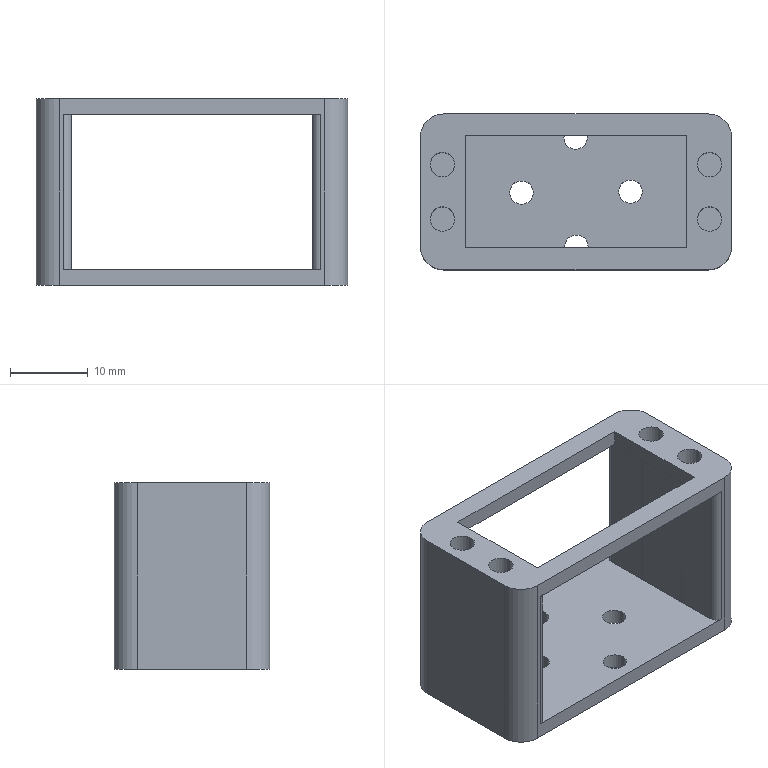Part | SolidWorks | features ICE 5, Fillet 2, Extrusion 1 | 1 solid | 42 faces | box 40 x 20 x 24 mm | volume 5034 mm3 | cylinder 24 | plane 18 | commonest cylinder face diameters 3 x8 3.15 x8 2 x4 6 x4
STEP:
#1=CARTESIAN_POINT('',(1.439,7.,-20.));
#2=VERTEX_POINT('',#1);
#3=CARTESIAN_POINT('',(-1.561,7.,-20.));
#4=VERTEX_POINT('',#3);
#5=CARTESIAN_POINT('',(-0.06094,7.,-20.));
#6=DIRECTION('',(0.,0.,-1.));
#7=DIRECTION('',(-1.,0.,0.));
#8=AXIS2_PLACEMENT_3D('',#5,#6,#7);
#9=CIRCLE('',#8,1.5);
#10=EDGE_CURVE('',#2,#4,#9,.T.);
#11=ORIENTED_EDGE('',*,*,#10,.F.);
#12=CARTESIAN_POINT('',(1.439,7.,-22.));
#13=VERTEX_POINT('',#12);
#14=CARTESIAN_POINT('',(1.439,7.,-20.));
#15=DIRECTION('',(0.,0.,-1.));
#16=VECTOR('',#15,1000.);
#17=LINE('',#14,#16);
#18=EDGE_CURVE('',#2,#13,#17,.T.);
#19=ORIENTED_EDGE('',*,*,#18,.T.);
#20=CARTESIAN_POINT('',(-1.561,7.,-22.));
#21=VERTEX_POINT('',#20);
#22=CARTESIAN_POINT('',(-0.06094,7.,-22.));
#23=DIRECTION('',(0.,0.,-1.));
#24=DIRECTION('',(-1.,0.,0.));
#25=AXIS2_PLACEMENT_3D('',#22,#23,#24);
#26=CIRCLE('',#25,1.5);
#27=EDGE_CURVE('',#13,#21,#26,.T.);
#28=ORIENTED_EDGE('',*,*,#27,.T.);
#29=CARTESIAN_POINT('',(-1.561,7.,-20.));
#30=DIRECTION('',(0.,0.,-1.));
#31=VECTOR('',#30,1000.);
#32=LINE('',#29,#31);
#33=EDGE_CURVE('',#4,#21,#32,.T.);
#34=ORIENTED_EDGE('',*,*,#33,.F.);
#35=EDGE_LOOP('',(#11,#19,#28,#34));
#36=FACE_OUTER_BOUND('',#35,.T.);
#37=CARTESIAN_POINT('',(-0.06094,7.,-20.));
#38=DIRECTION('',(0.,0.,-1.));
#39=DIRECTION('',(-1.,0.,0.));
#40=AXIS2_PLACEMENT_3D('',#37,#38,#39);
#41=CYLINDRICAL_SURFACE('',#40,1.5);
#42=ADVANCED_FACE('',(#36),#41,.F.);
#43=CARTESIAN_POINT('',(-5.5,-0.06094,-20.));
#44=VERTEX_POINT('',#43);
#45=CARTESIAN_POINT('',(-8.5,-0.06094,-20.));
#46=VERTEX_POINT('',#45);
#47=CARTESIAN_POINT('',(-7.,-0.06094,-20.));
#48=DIRECTION('',(0.,0.,-1.));
#49=DIRECTION('',(-1.,0.,0.));
#50=AXIS2_PLACEMENT_3D('',#47,#48,#49);
#51=CIRCLE('',#50,1.5);
#52=EDGE_CURVE('',#44,#46,#51,.T.);
#53=ORIENTED_EDGE('',*,*,#52,.F.);
#54=CARTESIAN_POINT('',(-5.5,-0.06094,-22.));
#55=VERTEX_POINT('',#54);
#56=CARTESIAN_POINT('',(-5.5,-0.06094,-20.));
#57=DIRECTION('',(0.,0.,-1.));
#58=VECTOR('',#57,1000.);
#59=LINE('',#56,#58);
#60=EDGE_CURVE('',#44,#55,#59,.T.);
#61=ORIENTED_EDGE('',*,*,#60,.T.);
#62=CARTESIAN_POINT('',(-8.5,-0.06094,-22.));
#63=VERTEX_POINT('',#62);
#64=CARTESIAN_POINT('',(-7.,-0.06094,-22.));
#65=DIRECTION('',(0.,0.,-1.));
#66=DIRECTION('',(-1.,0.,0.));
#67=AXIS2_PLACEMENT_3D('',#64,#65,#66);
#68=CIRCLE('',#67,1.5);
#69=EDGE_CURVE('',#55,#63,#68,.T.);
#70=ORIENTED_EDGE('',*,*,#69,.T.);
#71=CARTESIAN_POINT('',(-8.5,-0.06094,-20.));
#72=DIRECTION('',(0.,0.,-1.));
#73=VECTOR('',#72,1000.);
#74=LINE('',#71,#73);
#75=EDGE_CURVE('',#46,#63,#74,.T.);
#76=ORIENTED_EDGE('',*,*,#75,.F.);
#77=EDGE_LOOP('',(#53,#61,#70,#76));
#78=FACE_OUTER_BOUND('',#77,.T.);
#79=CARTESIAN_POINT('',(-7.,-0.06094,-20.));
#80=DIRECTION('',(0.,0.,-1.));
#81=DIRECTION('',(-1.,0.,0.));
#82=AXIS2_PLACEMENT_3D('',#79,#80,#81);
#83=CYLINDRICAL_SURFACE('',#82,1.5);
#84=ADVANCED_FACE('',(#78),#83,.F.);
#85=CARTESIAN_POINT('',(1.561,-7.,-20.));
#86=VERTEX_POINT('',#85);
#87=CARTESIAN_POINT('',(-1.439,-7.,-20.));
#88=VERTEX_POINT('',#87);
#89=CARTESIAN_POINT('',(0.06094,-7.,-20.));
#90=DIRECTION('',(0.,0.,-1.));
#91=DIRECTION('',(-1.,0.,0.));
#92=AXIS2_PLACEMENT_3D('',#89,#90,#91);
#93=CIRCLE('',#92,1.5);
#94=EDGE_CURVE('',#86,#88,#93,.T.);
#95=ORIENTED_EDGE('',*,*,#94,.F.);
#96=CARTESIAN_POINT('',(1.561,-7.,-22.));
#97=VERTEX_POINT('',#96);
#98=CARTESIAN_POINT('',(1.561,-7.,-20.));
#99=DIRECTION('',(0.,0.,-1.));
#100=VECTOR('',#99,1000.);
#101=LINE('',#98,#100);
#102=EDGE_CURVE('',#86,#97,#101,.T.);
#103=ORIENTED_EDGE('',*,*,#102,.T.);
#104=CARTESIAN_POINT('',(-1.439,-7.,-22.));
#105=VERTEX_POINT('',#104);
#106=CARTESIAN_POINT('',(0.06094,-7.,-22.));
#107=DIRECTION('',(0.,0.,-1.));
#108=DIRECTION('',(-1.,0.,0.));
#109=AXIS2_PLACEMENT_3D('',#106,#107,#108);
#110=CIRCLE('',#109,1.5);
#111=EDGE_CURVE('',#97,#105,#110,.T.);
#112=ORIENTED_EDGE('',*,*,#111,.T.);
#113=CARTESIAN_POINT('',(-1.439,-7.,-20.));
#114=DIRECTION('',(0.,0.,-1.));
#115=VECTOR('',#114,1000.);
#116=LINE('',#113,#115);
#117=EDGE_CURVE('',#88,#105,#116,.T.);
#118=ORIENTED_EDGE('',*,*,#117,.F.);
#119=EDGE_LOOP('',(#95,#103,#112,#118));
#120=FACE_OUTER_BOUND('',#119,.T.);
#121=CARTESIAN_POINT('',(0.06094,-7.,-20.));
#122=DIRECTION('',(0.,0.,-1.));
#123=DIRECTION('',(-1.,0.,0.));
#124=AXIS2_PLACEMENT_3D('',#121,#122,#123);
#125=CYLINDRICAL_SURFACE('',#124,1.5);
#126=ADVANCED_FACE('',(#120),#125,.F.);
#127=CARTESIAN_POINT('',(8.5,0.06094,-20.));
#128=VERTEX_POINT('',#127);
#129=CARTESIAN_POINT('',(5.5,0.06094,-20.));
#130=VERTEX_POINT('',#129);
#131=CARTESIAN_POINT('',(7.,0.06094,-20.));
#132=DIRECTION('',(0.,0.,-1.));
#133=DIRECTION('',(-1.,0.,0.));
#134=AXIS2_PLACEMENT_3D('',#131,#132,#133);
#135=CIRCLE('',#134,1.5);
#136=EDGE_CURVE('',#128,#130,#135,.T.);
#137=ORIENTED_EDGE('',*,*,#136,.F.);
#138=CARTESIAN_POINT('',(8.5,0.06094,-22.));
#139=VERTEX_POINT('',#138);
#140=CARTESIAN_POINT('',(8.5,0.06094,-20.));
#141=DIRECTION('',(0.,0.,-1.));
#142=VECTOR('',#141,1000.);
#143=LINE('',#140,#142);
#144=EDGE_CURVE('',#128,#139,#143,.T.);
#145=ORIENTED_EDGE('',*,*,#144,.T.);
#146=CARTESIAN_POINT('',(5.5,0.06094,-22.));
#147=VERTEX_POINT('',#146);
#148=CARTESIAN_POINT('',(7.,0.06094,-22.));
#149=DIRECTION('',(0.,0.,-1.));
#150=DIRECTION('',(-1.,0.,0.));
#151=AXIS2_PLACEMENT_3D('',#148,#149,#150);
#152=CIRCLE('',#151,1.5);
#153=EDGE_CURVE('',#139,#147,#152,.T.);
#154=ORIENTED_EDGE('',*,*,#153,.T.);
#155=CARTESIAN_POINT('',(5.5,0.06094,-20.));
#156=DIRECTION('',(0.,0.,-1.));
#157=VECTOR('',#156,1000.);
#158=LINE('',#155,#157);
#159=EDGE_CURVE('',#130,#147,#158,.T.);
#160=ORIENTED_EDGE('',*,*,#159,.F.);
#161=EDGE_LOOP('',(#137,#145,#154,#160));
#162=FACE_OUTER_BOUND('',#161,.T.);
#163=CARTESIAN_POINT('',(7.,0.06094,-20.));
#164=DIRECTION('',(0.,0.,-1.));
#165=DIRECTION('',(-1.,0.,0.));
#166=AXIS2_PLACEMENT_3D('',#163,#164,#165);
#167=CYLINDRICAL_SURFACE('',#166,1.5);
#168=ADVANCED_FACE('',(#162),#167,.F.);
#169=CARTESIAN_POINT('',(-18.725,-3.5,-20.));
#170=VERTEX_POINT('',#169);
#171=CARTESIAN_POINT('',(-15.575,-3.5,-20.));
#172=VERTEX_POINT('',#171);
#173=CARTESIAN_POINT('',(-17.15,-3.5,-20.));
#174=DIRECTION('',(0.,0.,1.));
#175=DIRECTION('',(-1.,0.,0.));
#176=AXIS2_PLACEMENT_3D('',#173,#174,#175);
#177=CIRCLE('',#176,1.575);
#178=EDGE_CURVE('',#170,#172,#177,.T.);
#179=ORIENTED_EDGE('',*,*,#178,.F.);
#180=CARTESIAN_POINT('',(-18.725,-3.5,2.));
#181=VERTEX_POINT('',#180);
#182=CARTESIAN_POINT('',(-18.725,-3.5,-4.));
#183=DIRECTION('',(0.,0.,1.));
#184=VECTOR('',#183,1000.);
#185=LINE('',#182,#184);
#186=EDGE_CURVE('',#170,#181,#185,.T.);
#187=ORIENTED_EDGE('',*,*,#186,.T.);
#188=CARTESIAN_POINT('',(-15.575,-3.5,2.));
#189=VERTEX_POINT('',#188);
#190=CARTESIAN_POINT('',(-17.15,-3.5,2.));
#191=DIRECTION('',(0.,0.,1.));
#192=DIRECTION('',(1.,0.,0.));
#193=AXIS2_PLACEMENT_3D('',#190,#191,#192);
#194=CIRCLE('',#193,1.575);
#195=EDGE_CURVE('',#181,#189,#194,.T.);
#196=ORIENTED_EDGE('',*,*,#195,.T.);
#197=CARTESIAN_POINT('',(-15.575,-3.5,-4.));
#198=DIRECTION('',(0.,0.,1.));
#199=VECTOR('',#198,1000.);
#200=LINE('',#197,#199);
#201=EDGE_CURVE('',#172,#189,#200,.T.);
#202=ORIENTED_EDGE('',*,*,#201,.F.);
#203=EDGE_LOOP('',(#179,#187,#196,#202));
#204=FACE_OUTER_BOUND('',#203,.T.);
#205=CARTESIAN_POINT('',(-17.15,-3.5,-4.));
#206=DIRECTION('',(0.,0.,1.));
#207=DIRECTION('',(1.,0.,0.));
#208=AXIS2_PLACEMENT_3D('',#205,#206,#207);
#209=CYLINDRICAL_SURFACE('',#208,1.575);
#210=ADVANCED_FACE('',(#204),#209,.F.);
#211=CARTESIAN_POINT('',(15.575,3.5,-20.));
#212=VERTEX_POINT('',#211);
#213=CARTESIAN_POINT('',(18.725,3.5,-20.));
#214=VERTEX_POINT('',#213);
#215=CARTESIAN_POINT('',(17.15,3.5,-20.));
#216=DIRECTION('',(0.,0.,1.));
#217=DIRECTION('',(-1.,0.,0.));
#218=AXIS2_PLACEMENT_3D('',#215,#216,#217);
#219=CIRCLE('',#218,1.575);
#220=EDGE_CURVE('',#212,#214,#219,.T.);
#221=ORIENTED_EDGE('',*,*,#220,.F.);
#222=CARTESIAN_POINT('',(15.575,3.5,2.));
#223=VERTEX_POINT('',#222);
#224=CARTESIAN_POINT('',(15.575,3.5,-4.));
#225=DIRECTION('',(0.,0.,1.));
#226=VECTOR('',#225,1000.);
#227=LINE('',#224,#226);
#228=EDGE_CURVE('',#212,#223,#227,.T.);
#229=ORIENTED_EDGE('',*,*,#228,.T.);
#230=CARTESIAN_POINT('',(18.725,3.5,2.));
#231=VERTEX_POINT('',#230);
#232=CARTESIAN_POINT('',(17.15,3.5,2.));
#233=DIRECTION('',(0.,0.,1.));
#234=DIRECTION('',(-1.,0.,0.));
#235=AXIS2_PLACEMENT_3D('',#232,#233,#234);
#236=CIRCLE('',#235,1.575);
#237=EDGE_CURVE('',#223,#231,#236,.T.);
#238=ORIENTED_EDGE('',*,*,#237,.T.);
#239=CARTESIAN_POINT('',(18.725,3.5,-4.));
#240=DIRECTION('',(0.,0.,1.));
#241=VECTOR('',#240,1000.);
#242=LINE('',#239,#241);
#243=EDGE_CURVE('',#214,#231,#242,.T.);
#244=ORIENTED_EDGE('',*,*,#243,.F.);
#245=EDGE_LOOP('',(#221,#229,#238,#244));
#246=FACE_OUTER_BOUND('',#245,.T.);
#247=CARTESIAN_POINT('',(17.15,3.5,-4.));
#248=DIRECTION('',(0.,0.,1.));
#249=DIRECTION('',(1.,0.,0.));
#250=AXIS2_PLACEMENT_3D('',#247,#248,#249);
#251=CYLINDRICAL_SURFACE('',#250,1.575);
#252=ADVANCED_FACE('',(#246),#251,.F.);
#253=CARTESIAN_POINT('',(15.575,-3.5,-20.));
#254=VERTEX_POINT('',#253);
#255=CARTESIAN_POINT('',(18.725,-3.5,-20.));
#256=VERTEX_POINT('',#255);
#257=CARTESIAN_POINT('',(17.15,-3.5,-20.));
#258=DIRECTION('',(0.,0.,1.));
#259=DIRECTION('',(-1.,0.,0.));
#260=AXIS2_PLACEMENT_3D('',#257,#258,#259);
#261=CIRCLE('',#260,1.575);
#262=EDGE_CURVE('',#254,#256,#261,.T.);
#263=ORIENTED_EDGE('',*,*,#262,.F.);
#264=CARTESIAN_POINT('',(15.575,-3.5,2.));
#265=VERTEX_POINT('',#264);
#266=CARTESIAN_POINT('',(15.575,-3.5,-4.));
#267=DIRECTION('',(0.,0.,1.));
#268=VECTOR('',#267,1000.);
#269=LINE('',#266,#268);
#270=EDGE_CURVE('',#254,#265,#269,.T.);
#271=ORIENTED_EDGE('',*,*,#270,.T.);
#272=CARTESIAN_POINT('',(18.725,-3.5,2.));
#273=VERTEX_POINT('',#272);
#274=CARTESIAN_POINT('',(17.15,-3.5,2.));
#275=DIRECTION('',(0.,0.,1.));
#276=DIRECTION('',(-1.,0.,0.));
#277=AXIS2_PLACEMENT_3D('',#274,#275,#276);
#278=CIRCLE('',#277,1.575);
#279=EDGE_CURVE('',#265,#273,#278,.T.);
#280=ORIENTED_EDGE('',*,*,#279,.T.);
#281=CARTESIAN_POINT('',(18.725,-3.5,-4.));
#282=DIRECTION('',(0.,0.,1.));
#283=VECTOR('',#282,1000.);
#284=LINE('',#281,#283);
#285=EDGE_CURVE('',#256,#273,#284,.T.);
#286=ORIENTED_EDGE('',*,*,#285,.F.);
#287=EDGE_LOOP('',(#263,#271,#280,#286));
#288=FACE_OUTER_BOUND('',#287,.T.);
#289=CARTESIAN_POINT('',(17.15,-3.5,-4.));
#290=DIRECTION('',(0.,0.,1.));
#291=DIRECTION('',(1.,0.,0.));
#292=AXIS2_PLACEMENT_3D('',#289,#290,#291);
#293=CYLINDRICAL_SURFACE('',#292,1.575);
#294=ADVANCED_FACE('',(#288),#293,.F.);
#295=CARTESIAN_POINT('',(-18.725,3.5,-20.));
#296=VERTEX_POINT('',#295);
#297=CARTESIAN_POINT('',(-15.575,3.5,-20.));
#298=VERTEX_POINT('',#297);
#299=CARTESIAN_POINT('',(-17.15,3.5,-20.));
#300=DIRECTION('',(0.,0.,1.));
#301=DIRECTION('',(-1.,0.,0.));
#302=AXIS2_PLACEMENT_3D('',#299,#300,#301);
#303=CIRCLE('',#302,1.575);
#304=EDGE_CURVE('',#296,#298,#303,.T.);
#305=ORIENTED_EDGE('',*,*,#304,.F.);
#306=CARTESIAN_POINT('',(-18.725,3.5,2.));
#307=VERTEX_POINT('',#306);
#308=CARTESIAN_POINT('',(-18.725,3.5,-4.));
#309=DIRECTION('',(0.,0.,1.));
#310=VECTOR('',#309,1000.);
#311=LINE('',#308,#310);
#312=EDGE_CURVE('',#296,#307,#311,.T.);
#313=ORIENTED_EDGE('',*,*,#312,.T.);
#314=CARTESIAN_POINT('',(-15.575,3.5,2.));
#315=VERTEX_POINT('',#314);
#316=CARTESIAN_POINT('',(-17.15,3.5,2.));
#317=DIRECTION('',(0.,0.,1.));
#318=DIRECTION('',(1.,0.,0.));
#319=AXIS2_PLACEMENT_3D('',#316,#317,#318);
#320=CIRCLE('',#319,1.575);
#321=EDGE_CURVE('',#307,#315,#320,.T.);
#322=ORIENTED_EDGE('',*,*,#321,.T.);
#323=CARTESIAN_POINT('',(-15.575,3.5,-4.));
#324=DIRECTION('',(0.,0.,1.));
#325=VECTOR('',#324,1000.);
#326=LINE('',#323,#325);
#327=EDGE_CURVE('',#298,#315,#326,.T.);
#328=ORIENTED_EDGE('',*,*,#327,.F.);
#329=EDGE_LOOP('',(#305,#313,#322,#328));
#330=FACE_OUTER_BOUND('',#329,.T.);
#331=CARTESIAN_POINT('',(-17.15,3.5,-4.));
#332=DIRECTION('',(0.,0.,1.));
#333=DIRECTION('',(1.,0.,0.));
#334=AXIS2_PLACEMENT_3D('',#331,#332,#333);
#335=CYLINDRICAL_SURFACE('',#334,1.575);
#336=ADVANCED_FACE('',(#330),#335,.F.);
#337=CARTESIAN_POINT('',(14.25,-7.2,0.));
#338=VERTEX_POINT('',#337);
#339=CARTESIAN_POINT('',(-14.25,-7.2,0.));
#340=VERTEX_POINT('',#339);
#341=CARTESIAN_POINT('',(0.,-7.2,0.));
#342=DIRECTION('',(-1.,0.,0.));
#343=VECTOR('',#342,1000.);
#344=LINE('',#341,#343);
#345=EDGE_CURVE('',#338,#340,#344,.T.);
#346=ORIENTED_EDGE('',*,*,#345,.F.);
#347=CARTESIAN_POINT('',(14.25,7.2,0.));
#348=VERTEX_POINT('',#347);
#349=CARTESIAN_POINT('',(14.25,0.,0.));
#350=DIRECTION('',(0.,-1.,0.));
#351=VECTOR('',#350,1000.);
#352=LINE('',#349,#351);
#353=EDGE_CURVE('',#348,#338,#352,.T.);
#354=ORIENTED_EDGE('',*,*,#353,.F.);
#355=CARTESIAN_POINT('',(-14.25,7.2,0.));
#356=VERTEX_POINT('',#355);
#357=CARTESIAN_POINT('',(0.,7.2,0.));
#358=DIRECTION('',(-1.,0.,0.));
#359=VECTOR('',#358,1000.);
#360=LINE('',#357,#359);
#361=EDGE_CURVE('',#348,#356,#360,.T.);
#362=ORIENTED_EDGE('',*,*,#361,.T.);
#363=CARTESIAN_POINT('',(-14.25,0.,0.));
#364=DIRECTION('',(0.,-1.,0.));
#365=VECTOR('',#364,1000.);
#366=LINE('',#363,#365);
#367=EDGE_CURVE('',#356,#340,#366,.T.);
#368=ORIENTED_EDGE('',*,*,#367,.T.);
#369=EDGE_LOOP('',(#346,#354,#362,#368));
#370=FACE_BOUND('',#369,.T.);
#371=CARTESIAN_POINT('',(16.5,10.,0.));
#372=VERTEX_POINT('',#371);
#373=CARTESIAN_POINT('',(-16.5,10.,0.));
#374=VERTEX_POINT('',#373);
#375=CARTESIAN_POINT('',(-20.,10.,0.));
#376=DIRECTION('',(-1.,0.,0.));
#377=VECTOR('',#376,1000.);
#378=LINE('',#375,#377);
#379=EDGE_CURVE('',#372,#374,#378,.T.);
#380=ORIENTED_EDGE('',*,*,#379,.F.);
#381=CARTESIAN_POINT('',(15.5,9.,0.));
#382=VERTEX_POINT('',#381);
#383=CARTESIAN_POINT('',(16.5,9.,0.));
#384=DIRECTION('',(0.,0.,1.));
#385=DIRECTION('',(-1.,0.,0.));
#386=AXIS2_PLACEMENT_3D('',#383,#384,#385);
#387=CIRCLE('',#386,1.);
#388=EDGE_CURVE('',#372,#382,#387,.T.);
#389=ORIENTED_EDGE('',*,*,#388,.T.);
#390=CARTESIAN_POINT('',(15.5,-9.,0.));
#391=VERTEX_POINT('',#390);
#392=CARTESIAN_POINT('',(15.5,0.,0.));
#393=DIRECTION('',(0.,1.,0.));
#394=VECTOR('',#393,1000.);
#395=LINE('',#392,#394);
#396=EDGE_CURVE('',#391,#382,#395,.T.);
#397=ORIENTED_EDGE('',*,*,#396,.F.);
#398=CARTESIAN_POINT('',(16.5,-10.,0.));
#399=VERTEX_POINT('',#398);
#400=CARTESIAN_POINT('',(16.5,-9.,0.));
#401=DIRECTION('',(0.,0.,1.));
#402=DIRECTION('',(-1.,0.,0.));
#403=AXIS2_PLACEMENT_3D('',#400,#401,#402);
#404=CIRCLE('',#403,1.);
#405=EDGE_CURVE('',#391,#399,#404,.T.);
#406=ORIENTED_EDGE('',*,*,#405,.T.);
#407=CARTESIAN_POINT('',(-16.5,-10.,0.));
#408=VERTEX_POINT('',#407);
#409=CARTESIAN_POINT('',(-20.,-10.,0.));
#410=DIRECTION('',(1.,0.,0.));
#411=VECTOR('',#410,1000.);
#412=LINE('',#409,#411);
#413=EDGE_CURVE('',#408,#399,#412,.T.);
#414=ORIENTED_EDGE('',*,*,#413,.F.);
#415=CARTESIAN_POINT('',(-15.5,-9.,0.));
#416=VERTEX_POINT('',#415);
#417=CARTESIAN_POINT('',(-16.5,-9.,0.));
#418=DIRECTION('',(0.,0.,1.));
#419=DIRECTION('',(-1.,0.,0.));
#420=AXIS2_PLACEMENT_3D('',#417,#418,#419);
#421=CIRCLE('',#420,1.);
#422=EDGE_CURVE('',#408,#416,#421,.T.);
#423=ORIENTED_EDGE('',*,*,#422,.T.);
#424=CARTESIAN_POINT('',(-15.5,9.,0.));
#425=VERTEX_POINT('',#424);
#426=CARTESIAN_POINT('',(-15.5,0.,0.));
#427=DIRECTION('',(0.,1.,0.));
#428=VECTOR('',#427,1000.);
#429=LINE('',#426,#428);
#430=EDGE_CURVE('',#416,#425,#429,.T.);
#431=ORIENTED_EDGE('',*,*,#430,.T.);
#432=CARTESIAN_POINT('',(-16.5,9.,0.));
#433=DIRECTION('',(0.,0.,1.));
#434=DIRECTION('',(-1.,0.,0.));
#435=AXIS2_PLACEMENT_3D('',#432,#433,#434);
#436=CIRCLE('',#435,1.);
#437=EDGE_CURVE('',#425,#374,#436,.T.);
#438=ORIENTED_EDGE('',*,*,#437,.T.);
#439=EDGE_LOOP('',(#380,#389,#397,#406,#414,#423,#431,#438));
#440=FACE_OUTER_BOUND('',#439,.T.);
#441=CARTESIAN_POINT('',(0.,0.,0.));
#442=DIRECTION('',(0.,0.,-1.));
#443=DIRECTION('',(-1.,0.,0.));
#444=AXIS2_PLACEMENT_3D('',#441,#442,#443);
#445=PLANE('',#444);
#446=ADVANCED_FACE('',(#370,#440),#445,.T.);
#447=CARTESIAN_POINT('',(20.,-7.,2.));
#448=VERTEX_POINT('',#447);
#449=CARTESIAN_POINT('',(20.,7.,2.));
#450=VERTEX_POINT('',#449);
#451=CARTESIAN_POINT('',(20.,-10.,2.));
#452=DIRECTION('',(0.,1.,0.));
#453=VECTOR('',#452,1000.);
#454=LINE('',#451,#453);
#455=EDGE_CURVE('',#448,#450,#454,.T.);
#456=ORIENTED_EDGE('',*,*,#455,.F.);
#457=CARTESIAN_POINT('',(20.,-7.,-22.));
#458=VERTEX_POINT('',#457);
#459=CARTESIAN_POINT('',(20.,-7.,2.));
#460=DIRECTION('',(0.,0.,-1.));
#461=VECTOR('',#460,1000.);
#462=LINE('',#459,#461);
#463=EDGE_CURVE('',#448,#458,#462,.T.);
#464=ORIENTED_EDGE('',*,*,#463,.T.);
#465=CARTESIAN_POINT('',(20.,7.,-22.));
#466=VERTEX_POINT('',#465);
#467=CARTESIAN_POINT('',(20.,10.,-22.));
#468=DIRECTION('',(0.,-1.,0.));
#469=VECTOR('',#468,1000.);
#470=LINE('',#467,#469);
#471=EDGE_CURVE('',#466,#458,#470,.T.);
#472=ORIENTED_EDGE('',*,*,#471,.F.);
#473=CARTESIAN_POINT('',(20.,7.,2.));
#474=DIRECTION('',(0.,0.,1.));
#475=VECTOR('',#474,1000.);
#476=LINE('',#473,#475);
#477=EDGE_CURVE('',#466,#450,#476,.T.);
#478=ORIENTED_EDGE('',*,*,#477,.T.);
#479=EDGE_LOOP('',(#456,#464,#472,#478));
#480=FACE_OUTER_BOUND('',#479,.T.);
#481=CARTESIAN_POINT('',(20.,-10.,2.));
#482=DIRECTION('',(-1.,0.,0.));
#483=DIRECTION('',(0.,0.,1.));
#484=AXIS2_PLACEMENT_3D('',#481,#482,#483);
#485=PLANE('',#484);
#486=ADVANCED_FACE('',(#480),#485,.F.);
#487=ORIENTED_EDGE('',*,*,#379,.T.);
#488=CARTESIAN_POINT('',(-16.5,10.,-20.));
#489=VERTEX_POINT('',#488);
#490=CARTESIAN_POINT('',(-16.5,10.,-20.));
#491=DIRECTION('',(0.,0.,-1.));
#492=VECTOR('',#491,1000.);
#493=LINE('',#490,#492);
#494=EDGE_CURVE('',#374,#489,#493,.T.);
#495=ORIENTED_EDGE('',*,*,#494,.T.);
#496=CARTESIAN_POINT('',(16.5,10.,-20.));
#497=VERTEX_POINT('',#496);
#498=CARTESIAN_POINT('',(20.,10.,-20.));
#499=DIRECTION('',(1.,0.,0.));
#500=VECTOR('',#499,1000.);
#501=LINE('',#498,#500);
#502=EDGE_CURVE('',#489,#497,#501,.T.);
#503=ORIENTED_EDGE('',*,*,#502,.T.);
#504=CARTESIAN_POINT('',(16.5,10.,2.));
#505=DIRECTION('',(0.,0.,1.));
#506=VECTOR('',#505,1000.);
#507=LINE('',#504,#506);
#508=EDGE_CURVE('',#497,#372,#507,.T.);
#509=ORIENTED_EDGE('',*,*,#508,.T.);
#510=EDGE_LOOP('',(#487,#495,#503,#509));
#511=FACE_BOUND('',#510,.T.);
#512=CARTESIAN_POINT('',(-17.,10.,-22.));
#513=VERTEX_POINT('',#512);
#514=CARTESIAN_POINT('',(17.,10.,-22.));
#515=VERTEX_POINT('',#514);
#516=CARTESIAN_POINT('',(20.,10.,-22.));
#517=DIRECTION('',(1.,0.,0.));
#518=VECTOR('',#517,1000.);
#519=LINE('',#516,#518);
#520=EDGE_CURVE('',#513,#515,#519,.T.);
#521=ORIENTED_EDGE('',*,*,#520,.F.);
#522=CARTESIAN_POINT('',(-17.,10.,2.));
#523=VERTEX_POINT('',#522);
#524=CARTESIAN_POINT('',(-17.,10.,2.));
#525=DIRECTION('',(0.,0.,1.));
#526=VECTOR('',#525,1000.);
#527=LINE('',#524,#526);
#528=EDGE_CURVE('',#513,#523,#527,.T.);
#529=ORIENTED_EDGE('',*,*,#528,.T.);
#530=CARTESIAN_POINT('',(17.,10.,2.));
#531=VERTEX_POINT('',#530);
#532=CARTESIAN_POINT('',(-20.,10.,2.));
#533=DIRECTION('',(-1.,0.,0.));
#534=VECTOR('',#533,1000.);
#535=LINE('',#532,#534);
#536=EDGE_CURVE('',#531,#523,#535,.T.);
#537=ORIENTED_EDGE('',*,*,#536,.F.);
#538=CARTESIAN_POINT('',(17.,10.,2.));
#539=DIRECTION('',(0.,0.,-1.));
#540=VECTOR('',#539,1000.);
#541=LINE('',#538,#540);
#542=EDGE_CURVE('',#531,#515,#541,.T.);
#543=ORIENTED_EDGE('',*,*,#542,.T.);
#544=EDGE_LOOP('',(#521,#529,#537,#543));
#545=FACE_OUTER_BOUND('',#544,.T.);
#546=CARTESIAN_POINT('',(-20.,10.,2.));
#547=DIRECTION('',(0.,-1.,0.));
#548=DIRECTION('',(0.,0.,-1.));
#549=AXIS2_PLACEMENT_3D('',#546,#547,#548);
#550=PLANE('',#549);
#551=ADVANCED_FACE('',(#511,#545),#550,.F.);
#552=CARTESIAN_POINT('',(-20.,7.,2.));
#553=VERTEX_POINT('',#552);
#554=CARTESIAN_POINT('',(-20.,-7.,2.));
#555=VERTEX_POINT('',#554);
#556=CARTESIAN_POINT('',(-20.,-10.,2.));
#557=DIRECTION('',(0.,-1.,0.));
#558=VECTOR('',#557,1000.);
#559=LINE('',#556,#558);
#560=EDGE_CURVE('',#553,#555,#559,.T.);
#561=ORIENTED_EDGE('',*,*,#560,.F.);
#562=CARTESIAN_POINT('',(-20.,7.,-22.));
#563=VERTEX_POINT('',#562);
#564=CARTESIAN_POINT('',(-20.,7.,2.));
#565=DIRECTION('',(0.,0.,-1.));
#566=VECTOR('',#565,1000.);
#567=LINE('',#564,#566);
#568=EDGE_CURVE('',#553,#563,#567,.T.);
#569=ORIENTED_EDGE('',*,*,#568,.T.);
#570=CARTESIAN_POINT('',(-20.,-7.,-22.));
#571=VERTEX_POINT('',#570);
#572=CARTESIAN_POINT('',(-20.,10.,-22.));
#573=DIRECTION('',(0.,1.,0.));
#574=VECTOR('',#573,1000.);
#575=LINE('',#572,#574);
#576=EDGE_CURVE('',#571,#563,#575,.T.);
#577=ORIENTED_EDGE('',*,*,#576,.F.);
#578=CARTESIAN_POINT('',(-20.,-7.,2.));
#579=DIRECTION('',(0.,0.,1.));
#580=VECTOR('',#579,1000.);
#581=LINE('',#578,#580);
#582=EDGE_CURVE('',#571,#555,#581,.T.);
#583=ORIENTED_EDGE('',*,*,#582,.T.);
#584=EDGE_LOOP('',(#561,#569,#577,#583));
#585=FACE_OUTER_BOUND('',#584,.T.);
#586=CARTESIAN_POINT('',(-20.,-10.,2.));
#587=DIRECTION('',(1.,0.,0.));
#588=DIRECTION('',(0.,0.,-1.));
#589=AXIS2_PLACEMENT_3D('',#586,#587,#588);
#590=PLANE('',#589);
#591=ADVANCED_FACE('',(#585),#590,.F.);
#592=CARTESIAN_POINT('',(-17.,-10.,2.));
#593=VERTEX_POINT('',#592);
#594=CARTESIAN_POINT('',(17.,-10.,2.));
#595=VERTEX_POINT('',#594);
#596=CARTESIAN_POINT('',(-20.,-10.,2.));
#597=DIRECTION('',(1.,0.,0.));
#598=VECTOR('',#597,1000.);
#599=LINE('',#596,#598);
#600=EDGE_CURVE('',#593,#595,#599,.T.);
#601=ORIENTED_EDGE('',*,*,#600,.F.);
#602=CARTESIAN_POINT('',(-17.,-10.,-22.));
#603=VERTEX_POINT('',#602);
#604=CARTESIAN_POINT('',(-17.,-10.,2.));
#605=DIRECTION('',(0.,0.,-1.));
#606=VECTOR('',#605,1000.);
#607=LINE('',#604,#606);
#608=EDGE_CURVE('',#593,#603,#607,.T.);
#609=ORIENTED_EDGE('',*,*,#608,.T.);
#610=CARTESIAN_POINT('',(17.,-10.,-22.));
#611=VERTEX_POINT('',#610);
#612=CARTESIAN_POINT('',(20.,-10.,-22.));
#613=DIRECTION('',(-1.,0.,0.));
#614=VECTOR('',#613,1000.);
#615=LINE('',#612,#614);
#616=EDGE_CURVE('',#611,#603,#615,.T.);
#617=ORIENTED_EDGE('',*,*,#616,.F.);
#618=CARTESIAN_POINT('',(17.,-10.,2.));
#619=DIRECTION('',(0.,0.,1.));
#620=VECTOR('',#619,1000.);
#621=LINE('',#618,#620);
#622=EDGE_CURVE('',#611,#595,#621,.T.);
#623=ORIENTED_EDGE('',*,*,#622,.T.);
#624=EDGE_LOOP('',(#601,#609,#617,#623));
#625=FACE_OUTER_BOUND('',#624,.T.);
#626=CARTESIAN_POINT('',(-16.5,-10.,-20.));
#627=VERTEX_POINT('',#626);
#628=CARTESIAN_POINT('',(-16.5,-10.,0.));
#629=DIRECTION('',(0.,0.,1.));
#630=VECTOR('',#629,1000.);
#631=LINE('',#628,#630);
#632=EDGE_CURVE('',#627,#408,#631,.T.);
#633=ORIENTED_EDGE('',*,*,#632,.T.);
#634=ORIENTED_EDGE('',*,*,#413,.T.);
#635=CARTESIAN_POINT('',(16.5,-10.,-20.));
#636=VERTEX_POINT('',#635);
#637=CARTESIAN_POINT('',(16.5,-10.,2.));
#638=DIRECTION('',(0.,0.,-1.));
#639=VECTOR('',#638,1000.);
#640=LINE('',#637,#639);
#641=EDGE_CURVE('',#399,#636,#640,.T.);
#642=ORIENTED_EDGE('',*,*,#641,.T.);
#643=CARTESIAN_POINT('',(20.,-10.,-20.));
#644=DIRECTION('',(-1.,0.,0.));
#645=VECTOR('',#644,1000.);
#646=LINE('',#643,#645);
#647=EDGE_CURVE('',#636,#627,#646,.T.);
#648=ORIENTED_EDGE('',*,*,#647,.T.);
#649=EDGE_LOOP('',(#633,#634,#642,#648));
#650=FACE_BOUND('',#649,.T.);
#651=CARTESIAN_POINT('',(-20.,-10.,2.));
#652=DIRECTION('',(0.,1.,0.));
#653=DIRECTION('',(0.,0.,1.));
#654=AXIS2_PLACEMENT_3D('',#651,#652,#653);
#655=PLANE('',#654);
#656=ADVANCED_FACE('',(#625,#650),#655,.F.);
#657=CARTESIAN_POINT('',(-17.15,-3.5,2.));
#658=DIRECTION('',(0.,0.,1.));
#659=DIRECTION('',(1.,0.,0.));
#660=AXIS2_PLACEMENT_3D('',#657,#658,#659);
#661=CIRCLE('',#660,1.575);
#662=EDGE_CURVE('',#189,#181,#661,.T.);
#663=ORIENTED_EDGE('',*,*,#662,.F.);
#664=ORIENTED_EDGE('',*,*,#195,.F.);
#665=EDGE_LOOP('',(#663,#664));
#666=FACE_BOUND('',#665,.T.);
#667=CARTESIAN_POINT('',(17.15,3.5,2.));
#668=DIRECTION('',(0.,0.,1.));
#669=DIRECTION('',(-1.,0.,0.));
#670=AXIS2_PLACEMENT_3D('',#667,#668,#669);
#671=CIRCLE('',#670,1.575);
#672=EDGE_CURVE('',#231,#223,#671,.T.);
#673=ORIENTED_EDGE('',*,*,#672,.F.);
#674=ORIENTED_EDGE('',*,*,#237,.F.);
#675=EDGE_LOOP('',(#673,#674));
#676=FACE_BOUND('',#675,.T.);
#677=CARTESIAN_POINT('',(17.15,-3.5,2.));
#678=DIRECTION('',(0.,0.,1.));
#679=DIRECTION('',(-1.,0.,0.));
#680=AXIS2_PLACEMENT_3D('',#677,#678,#679);
#681=CIRCLE('',#680,1.575);
#682=EDGE_CURVE('',#273,#265,#681,.T.);
#683=ORIENTED_EDGE('',*,*,#682,.F.);
#684=ORIENTED_EDGE('',*,*,#279,.F.);
#685=EDGE_LOOP('',(#683,#684));
#686=FACE_BOUND('',#685,.T.);
#687=CARTESIAN_POINT('',(-17.15,3.5,2.));
#688=DIRECTION('',(0.,0.,1.));
#689=DIRECTION('',(1.,0.,0.));
#690=AXIS2_PLACEMENT_3D('',#687,#688,#689);
#691=CIRCLE('',#690,1.575);
#692=EDGE_CURVE('',#315,#307,#691,.T.);
#693=ORIENTED_EDGE('',*,*,#692,.F.);
#694=ORIENTED_EDGE('',*,*,#321,.F.);
#695=EDGE_LOOP('',(#693,#694));
#696=FACE_BOUND('',#695,.T.);
#697=CARTESIAN_POINT('',(14.25,-7.2,2.));
#698=VERTEX_POINT('',#697);
#699=CARTESIAN_POINT('',(14.25,7.2,2.));
#700=VERTEX_POINT('',#699);
#701=CARTESIAN_POINT('',(14.25,-7.2,2.));
#702=DIRECTION('',(0.,1.,0.));
#703=VECTOR('',#702,1000.);
#704=LINE('',#701,#703);
#705=EDGE_CURVE('',#698,#700,#704,.T.);
#706=ORIENTED_EDGE('',*,*,#705,.F.);
#707=CARTESIAN_POINT('',(-14.25,-7.2,2.));
#708=VERTEX_POINT('',#707);
#709=CARTESIAN_POINT('',(-14.25,-7.2,2.));
#710=DIRECTION('',(1.,0.,0.));
#711=VECTOR('',#710,1000.);
#712=LINE('',#709,#711);
#713=EDGE_CURVE('',#708,#698,#712,.T.);
#714=ORIENTED_EDGE('',*,*,#713,.F.);
#715=CARTESIAN_POINT('',(-14.25,7.2,2.));
#716=VERTEX_POINT('',#715);
#717=CARTESIAN_POINT('',(-14.25,-7.2,2.));
#718=DIRECTION('',(0.,1.,0.));
#719=VECTOR('',#718,1000.);
#720=LINE('',#717,#719);
#721=EDGE_CURVE('',#708,#716,#720,.T.);
#722=ORIENTED_EDGE('',*,*,#721,.T.);
#723=CARTESIAN_POINT('',(-14.25,7.2,2.));
#724=DIRECTION('',(1.,0.,0.));
#725=VECTOR('',#724,1000.);
#726=LINE('',#723,#725);
#727=EDGE_CURVE('',#716,#700,#726,.T.);
#728=ORIENTED_EDGE('',*,*,#727,.T.);
#729=EDGE_LOOP('',(#706,#714,#722,#728));
#730=FACE_BOUND('',#729,.T.);
#731=ORIENTED_EDGE('',*,*,#536,.T.);
#732=CARTESIAN_POINT('',(-17.,7.,2.));
#733=DIRECTION('',(0.,0.,1.));
#734=DIRECTION('',(-1.,0.,0.));
#735=AXIS2_PLACEMENT_3D('',#732,#733,#734);
#736=CIRCLE('',#735,3.);
#737=EDGE_CURVE('',#523,#553,#736,.T.);
#738=ORIENTED_EDGE('',*,*,#737,.T.);
#739=ORIENTED_EDGE('',*,*,#560,.T.);
#740=CARTESIAN_POINT('',(-17.,-7.,2.));
#741=DIRECTION('',(0.,0.,1.));
#742=DIRECTION('',(-1.,0.,0.));
#743=AXIS2_PLACEMENT_3D('',#740,#741,#742);
#744=CIRCLE('',#743,3.);
#745=EDGE_CURVE('',#555,#593,#744,.T.);
#746=ORIENTED_EDGE('',*,*,#745,.T.);
#747=ORIENTED_EDGE('',*,*,#600,.T.);
#748=CARTESIAN_POINT('',(17.,-7.,2.));
#749=DIRECTION('',(0.,0.,1.));
#750=DIRECTION('',(-1.,0.,0.));
#751=AXIS2_PLACEMENT_3D('',#748,#749,#750);
#752=CIRCLE('',#751,3.);
#753=EDGE_CURVE('',#595,#448,#752,.T.);
#754=ORIENTED_EDGE('',*,*,#753,.T.);
#755=ORIENTED_EDGE('',*,*,#455,.T.);
#756=CARTESIAN_POINT('',(17.,7.,2.));
#757=DIRECTION('',(0.,0.,1.));
#758=DIRECTION('',(-1.,0.,0.));
#759=AXIS2_PLACEMENT_3D('',#756,#757,#758);
#760=CIRCLE('',#759,3.);
#761=EDGE_CURVE('',#450,#531,#760,.T.);
#762=ORIENTED_EDGE('',*,*,#761,.T.);
#763=EDGE_LOOP('',(#731,#738,#739,#746,#747,#754,#755,#762));
#764=FACE_OUTER_BOUND('',#763,.T.);
#765=CARTESIAN_POINT('',(0.,0.,2.));
#766=DIRECTION('',(0.,0.,-1.));
#767=DIRECTION('',(-1.,0.,0.));
#768=AXIS2_PLACEMENT_3D('',#765,#766,#767);
#769=PLANE('',#768);
#770=ADVANCED_FACE('',(#666,#676,#686,#696,#730,#764),#769,.F.);
#771=ORIENTED_EDGE('',*,*,#345,.T.);
#772=CARTESIAN_POINT('',(-14.25,-7.2,-4.));
#773=DIRECTION('',(0.,0.,1.));
#774=VECTOR('',#773,1000.);
#775=LINE('',#772,#774);
#776=EDGE_CURVE('',#340,#708,#775,.T.);
#777=ORIENTED_EDGE('',*,*,#776,.T.);
#778=ORIENTED_EDGE('',*,*,#713,.T.);
#779=CARTESIAN_POINT('',(14.25,-7.2,-4.));
#780=DIRECTION('',(0.,0.,1.));
#781=VECTOR('',#780,1000.);
#782=LINE('',#779,#781);
#783=EDGE_CURVE('',#338,#698,#782,.T.);
#784=ORIENTED_EDGE('',*,*,#783,.F.);
#785=EDGE_LOOP('',(#771,#777,#778,#784));
#786=FACE_OUTER_BOUND('',#785,.T.);
#787=CARTESIAN_POINT('',(-14.25,-7.2,-4.));
#788=DIRECTION('',(0.,-1.,0.));
#789=DIRECTION('',(0.,0.,-1.));
#790=AXIS2_PLACEMENT_3D('',#787,#788,#789);
#791=PLANE('',#790);
#792=ADVANCED_FACE('',(#786),#791,.F.);
#793=CARTESIAN_POINT('',(-14.25,7.2,-4.));
#794=DIRECTION('',(0.,0.,1.));
#795=VECTOR('',#794,1000.);
#796=LINE('',#793,#795);
#797=EDGE_CURVE('',#356,#716,#796,.T.);
#798=ORIENTED_EDGE('',*,*,#797,.T.);
#799=ORIENTED_EDGE('',*,*,#721,.F.);
#800=ORIENTED_EDGE('',*,*,#776,.F.);
#801=ORIENTED_EDGE('',*,*,#367,.F.);
#802=EDGE_LOOP('',(#798,#799,#800,#801));
#803=FACE_OUTER_BOUND('',#802,.T.);
#804=CARTESIAN_POINT('',(-14.25,-7.2,-4.));
#805=DIRECTION('',(1.,0.,0.));
#806=DIRECTION('',(0.,0.,-1.));
#807=AXIS2_PLACEMENT_3D('',#804,#805,#806);
#808=PLANE('',#807);
#809=ADVANCED_FACE('',(#803),#808,.T.);
#810=CARTESIAN_POINT('',(14.25,7.2,-4.));
#811=DIRECTION('',(0.,0.,1.));
#812=VECTOR('',#811,1000.);
#813=LINE('',#810,#812);
#814=EDGE_CURVE('',#348,#700,#813,.T.);
#815=ORIENTED_EDGE('',*,*,#814,.T.);
#816=ORIENTED_EDGE('',*,*,#727,.F.);
#817=ORIENTED_EDGE('',*,*,#797,.F.);
#818=ORIENTED_EDGE('',*,*,#361,.F.);
#819=EDGE_LOOP('',(#815,#816,#817,#818));
#820=FACE_OUTER_BOUND('',#819,.T.);
#821=CARTESIAN_POINT('',(-14.25,7.2,-4.));
#822=DIRECTION('',(0.,-1.,0.));
#823=DIRECTION('',(0.,0.,-1.));
#824=AXIS2_PLACEMENT_3D('',#821,#822,#823);
#825=PLANE('',#824);
#826=ADVANCED_FACE('',(#820),#825,.T.);
#827=ORIENTED_EDGE('',*,*,#353,.T.);
#828=ORIENTED_EDGE('',*,*,#783,.T.);
#829=ORIENTED_EDGE('',*,*,#705,.T.);
#830=ORIENTED_EDGE('',*,*,#814,.F.);
#831=EDGE_LOOP('',(#827,#828,#829,#830));
#832=FACE_OUTER_BOUND('',#831,.T.);
#833=CARTESIAN_POINT('',(14.25,-7.2,-4.));
#834=DIRECTION('',(1.,0.,0.));
#835=DIRECTION('',(0.,0.,-1.));
#836=AXIS2_PLACEMENT_3D('',#833,#834,#835);
#837=PLANE('',#836);
#838=ADVANCED_FACE('',(#832),#837,.F.);
#839=ORIENTED_EDGE('',*,*,#312,.F.);
#840=CARTESIAN_POINT('',(-17.15,3.5,-20.));
#841=DIRECTION('',(0.,0.,1.));
#842=DIRECTION('',(-1.,0.,0.));
#843=AXIS2_PLACEMENT_3D('',#840,#841,#842);
#844=CIRCLE('',#843,1.575);
#845=EDGE_CURVE('',#298,#296,#844,.T.);
#846=ORIENTED_EDGE('',*,*,#845,.F.);
#847=ORIENTED_EDGE('',*,*,#327,.T.);
#848=ORIENTED_EDGE('',*,*,#692,.T.);
#849=EDGE_LOOP('',(#839,#846,#847,#848));
#850=FACE_OUTER_BOUND('',#849,.T.);
#851=CARTESIAN_POINT('',(-17.15,3.5,-4.));
#852=DIRECTION('',(0.,0.,1.));
#853=DIRECTION('',(1.,0.,0.));
#854=AXIS2_PLACEMENT_3D('',#851,#852,#853);
#855=CYLINDRICAL_SURFACE('',#854,1.575);
#856=ADVANCED_FACE('',(#850),#855,.F.);
#857=ORIENTED_EDGE('',*,*,#270,.F.);
#858=CARTESIAN_POINT('',(17.15,-3.5,-20.));
#859=DIRECTION('',(0.,0.,1.));
#860=DIRECTION('',(-1.,0.,0.));
#861=AXIS2_PLACEMENT_3D('',#858,#859,#860);
#862=CIRCLE('',#861,1.575);
#863=EDGE_CURVE('',#256,#254,#862,.T.);
#864=ORIENTED_EDGE('',*,*,#863,.F.);
#865=ORIENTED_EDGE('',*,*,#285,.T.);
#866=ORIENTED_EDGE('',*,*,#682,.T.);
#867=EDGE_LOOP('',(#857,#864,#865,#866));
#868=FACE_OUTER_BOUND('',#867,.T.);
#869=CARTESIAN_POINT('',(17.15,-3.5,-4.));
#870=DIRECTION('',(0.,0.,1.));
#871=DIRECTION('',(1.,0.,0.));
#872=AXIS2_PLACEMENT_3D('',#869,#870,#871);
#873=CYLINDRICAL_SURFACE('',#872,1.575);
#874=ADVANCED_FACE('',(#868),#873,.F.);
#875=ORIENTED_EDGE('',*,*,#228,.F.);
#876=CARTESIAN_POINT('',(17.15,3.5,-20.));
#877=DIRECTION('',(0.,0.,1.));
#878=DIRECTION('',(-1.,0.,0.));
#879=AXIS2_PLACEMENT_3D('',#876,#877,#878);
#880=CIRCLE('',#879,1.575);
#881=EDGE_CURVE('',#214,#212,#880,.T.);
#882=ORIENTED_EDGE('',*,*,#881,.F.);
#883=ORIENTED_EDGE('',*,*,#243,.T.);
#884=ORIENTED_EDGE('',*,*,#672,.T.);
#885=EDGE_LOOP('',(#875,#882,#883,#884));
#886=FACE_OUTER_BOUND('',#885,.T.);
#887=CARTESIAN_POINT('',(17.15,3.5,-4.));
#888=DIRECTION('',(0.,0.,1.));
#889=DIRECTION('',(1.,0.,0.));
#890=AXIS2_PLACEMENT_3D('',#887,#888,#889);
#891=CYLINDRICAL_SURFACE('',#890,1.575);
#892=ADVANCED_FACE('',(#886),#891,.F.);
#893=ORIENTED_EDGE('',*,*,#186,.F.);
#894=CARTESIAN_POINT('',(-17.15,-3.5,-20.));
#895=DIRECTION('',(0.,0.,1.));
#896=DIRECTION('',(-1.,0.,0.));
#897=AXIS2_PLACEMENT_3D('',#894,#895,#896);
#898=CIRCLE('',#897,1.575);
#899=EDGE_CURVE('',#172,#170,#898,.T.);
#900=ORIENTED_EDGE('',*,*,#899,.F.);
#901=ORIENTED_EDGE('',*,*,#201,.T.);
#902=ORIENTED_EDGE('',*,*,#662,.T.);
#903=EDGE_LOOP('',(#893,#900,#901,#902));
#904=FACE_OUTER_BOUND('',#903,.T.);
#905=CARTESIAN_POINT('',(-17.15,-3.5,-4.));
#906=DIRECTION('',(0.,0.,1.));
#907=DIRECTION('',(1.,0.,0.));
#908=AXIS2_PLACEMENT_3D('',#905,#906,#907);
#909=CYLINDRICAL_SURFACE('',#908,1.575);
#910=ADVANCED_FACE('',(#904),#909,.F.);
#911=ORIENTED_EDGE('',*,*,#430,.F.);
#912=CARTESIAN_POINT('',(-15.5,-9.,-20.));
#913=VERTEX_POINT('',#912);
#914=CARTESIAN_POINT('',(-15.5,-9.,-20.));
#915=DIRECTION('',(0.,0.,-1.));
#916=VECTOR('',#915,1000.);
#917=LINE('',#914,#916);
#918=EDGE_CURVE('',#416,#913,#917,.T.);
#919=ORIENTED_EDGE('',*,*,#918,.T.);
#920=CARTESIAN_POINT('',(-15.5,9.,-20.));
#921=VERTEX_POINT('',#920);
#922=CARTESIAN_POINT('',(-15.5,0.,-20.));
#923=DIRECTION('',(0.,1.,0.));
#924=VECTOR('',#923,1000.);
#925=LINE('',#922,#924);
#926=EDGE_CURVE('',#913,#921,#925,.T.);
#927=ORIENTED_EDGE('',*,*,#926,.T.);
#928=CARTESIAN_POINT('',(-15.5,9.,0.));
#929=DIRECTION('',(0.,0.,1.));
#930=VECTOR('',#929,1000.);
#931=LINE('',#928,#930);
#932=EDGE_CURVE('',#921,#425,#931,.T.);
#933=ORIENTED_EDGE('',*,*,#932,.T.);
#934=EDGE_LOOP('',(#911,#919,#927,#933));
#935=FACE_OUTER_BOUND('',#934,.T.);
#936=CARTESIAN_POINT('',(-15.5,0.,-20.));
#937=DIRECTION('',(1.,0.,0.));
#938=DIRECTION('',(0.,0.,-1.));
#939=AXIS2_PLACEMENT_3D('',#936,#937,#938);
#940=PLANE('',#939);
#941=ADVANCED_FACE('',(#935),#940,.T.);
#942=ORIENTED_EDGE('',*,*,#396,.T.);
#943=CARTESIAN_POINT('',(15.5,9.,-20.));
#944=VERTEX_POINT('',#943);
#945=CARTESIAN_POINT('',(15.5,9.,-20.));
#946=DIRECTION('',(0.,0.,-1.));
#947=VECTOR('',#946,1000.);
#948=LINE('',#945,#947);
#949=EDGE_CURVE('',#382,#944,#948,.T.);
#950=ORIENTED_EDGE('',*,*,#949,.T.);
#951=CARTESIAN_POINT('',(15.5,-9.,-20.));
#952=VERTEX_POINT('',#951);
#953=CARTESIAN_POINT('',(15.5,0.,-20.));
#954=DIRECTION('',(0.,1.,0.));
#955=VECTOR('',#954,1000.);
#956=LINE('',#953,#955);
#957=EDGE_CURVE('',#952,#944,#956,.T.);
#958=ORIENTED_EDGE('',*,*,#957,.F.);
#959=CARTESIAN_POINT('',(15.5,-9.,-20.));
#960=DIRECTION('',(0.,0.,1.));
#961=VECTOR('',#960,1000.);
#962=LINE('',#959,#961);
#963=EDGE_CURVE('',#952,#391,#962,.T.);
#964=ORIENTED_EDGE('',*,*,#963,.T.);
#965=EDGE_LOOP('',(#942,#950,#958,#964));
#966=FACE_OUTER_BOUND('',#965,.T.);
#967=CARTESIAN_POINT('',(15.5,0.,-20.));
#968=DIRECTION('',(1.,0.,0.));
#969=DIRECTION('',(0.,1.,0.));
#970=AXIS2_PLACEMENT_3D('',#967,#968,#969);
#971=PLANE('',#970);
#972=ADVANCED_FACE('',(#966),#971,.F.);
#973=CARTESIAN_POINT('',(-0.06094,7.,-22.));
#974=DIRECTION('',(0.,0.,-1.));
#975=DIRECTION('',(-1.,0.,0.));
#976=AXIS2_PLACEMENT_3D('',#973,#974,#975);
#977=CIRCLE('',#976,1.5);
#978=EDGE_CURVE('',#21,#13,#977,.T.);
#979=ORIENTED_EDGE('',*,*,#978,.F.);
#980=ORIENTED_EDGE('',*,*,#27,.F.);
#981=EDGE_LOOP('',(#979,#980));
#982=FACE_BOUND('',#981,.T.);
#983=CARTESIAN_POINT('',(-7.,-0.06094,-22.));
#984=DIRECTION('',(0.,0.,-1.));
#985=DIRECTION('',(-1.,0.,0.));
#986=AXIS2_PLACEMENT_3D('',#983,#984,#985);
#987=CIRCLE('',#986,1.5);
#988=EDGE_CURVE('',#63,#55,#987,.T.);
#989=ORIENTED_EDGE('',*,*,#988,.F.);
#990=ORIENTED_EDGE('',*,*,#69,.F.);
#991=EDGE_LOOP('',(#989,#990));
#992=FACE_BOUND('',#991,.T.);
#993=CARTESIAN_POINT('',(0.06094,-7.,-22.));
#994=DIRECTION('',(0.,0.,-1.));
#995=DIRECTION('',(-1.,0.,0.));
#996=AXIS2_PLACEMENT_3D('',#993,#994,#995);
#997=CIRCLE('',#996,1.5);
#998=EDGE_CURVE('',#105,#97,#997,.T.);
#999=ORIENTED_EDGE('',*,*,#998,.F.);
#1000=ORIENTED_EDGE('',*,*,#111,.F.);
#1001=EDGE_LOOP('',(#999,#1000));
#1002=FACE_BOUND('',#1001,.T.);
#1003=CARTESIAN_POINT('',(7.,0.06094,-22.));
#1004=DIRECTION('',(0.,0.,-1.));
#1005=DIRECTION('',(-1.,0.,0.));
#1006=AXIS2_PLACEMENT_3D('',#1003,#1004,#1005);
#1007=CIRCLE('',#1006,1.5);
#1008=EDGE_CURVE('',#147,#139,#1007,.T.);
#1009=ORIENTED_EDGE('',*,*,#1008,.F.);
#1010=ORIENTED_EDGE('',*,*,#153,.F.);
#1011=EDGE_LOOP('',(#1009,#1010));
#1012=FACE_BOUND('',#1011,.T.);
#1013=ORIENTED_EDGE('',*,*,#576,.T.);
#1014=CARTESIAN_POINT('',(-17.,7.,-22.));
#1015=DIRECTION('',(0.,0.,-1.));
#1016=DIRECTION('',(-1.,0.,0.));
#1017=AXIS2_PLACEMENT_3D('',#1014,#1015,#1016);
#1018=CIRCLE('',#1017,3.);
#1019=EDGE_CURVE('',#563,#513,#1018,.T.);
#1020=ORIENTED_EDGE('',*,*,#1019,.T.);
#1021=ORIENTED_EDGE('',*,*,#520,.T.);
#1022=CARTESIAN_POINT('',(17.,7.,-22.));
#1023=DIRECTION('',(0.,0.,-1.));
#1024=DIRECTION('',(-1.,0.,0.));
#1025=AXIS2_PLACEMENT_3D('',#1022,#1023,#1024);
#1026=CIRCLE('',#1025,3.);
#1027=EDGE_CURVE('',#515,#466,#1026,.T.);
#1028=ORIENTED_EDGE('',*,*,#1027,.T.);
#1029=ORIENTED_EDGE('',*,*,#471,.T.);
#1030=CARTESIAN_POINT('',(17.,-7.,-22.));
#1031=DIRECTION('',(0.,0.,-1.));
#1032=DIRECTION('',(-1.,0.,0.));
#1033=AXIS2_PLACEMENT_3D('',#1030,#1031,#1032);
#1034=CIRCLE('',#1033,3.);
#1035=EDGE_CURVE('',#458,#611,#1034,.T.);
#1036=ORIENTED_EDGE('',*,*,#1035,.T.);
#1037=ORIENTED_EDGE('',*,*,#616,.T.);
#1038=CARTESIAN_POINT('',(-17.,-7.,-22.));
#1039=DIRECTION('',(0.,0.,-1.));
#1040=DIRECTION('',(-1.,0.,0.));
#1041=AXIS2_PLACEMENT_3D('',#1038,#1039,#1040);
#1042=CIRCLE('',#1041,3.);
#1043=EDGE_CURVE('',#603,#571,#1042,.T.);
#1044=ORIENTED_EDGE('',*,*,#1043,.T.);
#1045=EDGE_LOOP('',(#1013,#1020,#1021,#1028,#1029,#1036,#1037,#1044));
#1046=FACE_OUTER_BOUND('',#1045,.T.);
#1047=CARTESIAN_POINT('',(0.,0.,-22.));
#1048=DIRECTION('',(0.,0.,-1.));
#1049=DIRECTION('',(-1.,0.,0.));
#1050=AXIS2_PLACEMENT_3D('',#1047,#1048,#1049);
#1051=PLANE('',#1050);
#1052=ADVANCED_FACE('',(#982,#992,#1002,#1012,#1046),#1051,.T.);
#1053=CARTESIAN_POINT('',(-0.06094,7.,-20.));
#1054=DIRECTION('',(0.,0.,-1.));
#1055=DIRECTION('',(-1.,0.,0.));
#1056=AXIS2_PLACEMENT_3D('',#1053,#1054,#1055);
#1057=CIRCLE('',#1056,1.5);
#1058=EDGE_CURVE('',#4,#2,#1057,.T.);
#1059=ORIENTED_EDGE('',*,*,#1058,.T.);
#1060=ORIENTED_EDGE('',*,*,#10,.T.);
#1061=EDGE_LOOP('',(#1059,#1060));
#1062=FACE_BOUND('',#1061,.T.);
#1063=CARTESIAN_POINT('',(-7.,-0.06094,-20.));
#1064=DIRECTION('',(0.,0.,-1.));
#1065=DIRECTION('',(-1.,0.,0.));
#1066=AXIS2_PLACEMENT_3D('',#1063,#1064,#1065);
#1067=CIRCLE('',#1066,1.5);
#1068=EDGE_CURVE('',#46,#44,#1067,.T.);
#1069=ORIENTED_EDGE('',*,*,#1068,.T.);
#1070=ORIENTED_EDGE('',*,*,#52,.T.);
#1071=EDGE_LOOP('',(#1069,#1070));
#1072=FACE_BOUND('',#1071,.T.);
#1073=CARTESIAN_POINT('',(0.06094,-7.,-20.));
#1074=DIRECTION('',(0.,0.,-1.));
#1075=DIRECTION('',(-1.,0.,0.));
#1076=AXIS2_PLACEMENT_3D('',#1073,#1074,#1075);
#1077=CIRCLE('',#1076,1.5);
#1078=EDGE_CURVE('',#88,#86,#1077,.T.);
#1079=ORIENTED_EDGE('',*,*,#1078,.T.);
#1080=ORIENTED_EDGE('',*,*,#94,.T.);
#1081=EDGE_LOOP('',(#1079,#1080));
#1082=FACE_BOUND('',#1081,.T.);
#1083=CARTESIAN_POINT('',(7.,0.06094,-20.));
#1084=DIRECTION('',(0.,0.,-1.));
#1085=DIRECTION('',(-1.,0.,0.));
#1086=AXIS2_PLACEMENT_3D('',#1083,#1084,#1085);
#1087=CIRCLE('',#1086,1.5);
#1088=EDGE_CURVE('',#130,#128,#1087,.T.);
#1089=ORIENTED_EDGE('',*,*,#1088,.T.);
#1090=ORIENTED_EDGE('',*,*,#136,.T.);
#1091=EDGE_LOOP('',(#1089,#1090));
#1092=FACE_BOUND('',#1091,.T.);
#1093=ORIENTED_EDGE('',*,*,#926,.F.);
#1094=CARTESIAN_POINT('',(-16.5,-9.,-20.));
#1095=DIRECTION('',(0.,0.,-1.));
#1096=DIRECTION('',(-1.,0.,0.));
#1097=AXIS2_PLACEMENT_3D('',#1094,#1095,#1096);
#1098=CIRCLE('',#1097,1.);
#1099=EDGE_CURVE('',#913,#627,#1098,.T.);
#1100=ORIENTED_EDGE('',*,*,#1099,.T.);
#1101=ORIENTED_EDGE('',*,*,#647,.F.);
#1102=CARTESIAN_POINT('',(16.5,-9.,-20.));
#1103=DIRECTION('',(0.,0.,-1.));
#1104=DIRECTION('',(-1.,0.,0.));
#1105=AXIS2_PLACEMENT_3D('',#1102,#1103,#1104);
#1106=CIRCLE('',#1105,1.);
#1107=EDGE_CURVE('',#636,#952,#1106,.T.);
#1108=ORIENTED_EDGE('',*,*,#1107,.T.);
#1109=ORIENTED_EDGE('',*,*,#957,.T.);
#1110=CARTESIAN_POINT('',(16.5,9.,-20.));
#1111=DIRECTION('',(0.,0.,-1.));
#1112=DIRECTION('',(-1.,0.,0.));
#1113=AXIS2_PLACEMENT_3D('',#1110,#1111,#1112);
#1114=CIRCLE('',#1113,1.);
#1115=EDGE_CURVE('',#944,#497,#1114,.T.);
#1116=ORIENTED_EDGE('',*,*,#1115,.T.);
#1117=ORIENTED_EDGE('',*,*,#502,.F.);
#1118=CARTESIAN_POINT('',(-16.5,9.,-20.));
#1119=DIRECTION('',(0.,0.,-1.));
#1120=DIRECTION('',(-1.,0.,0.));
#1121=AXIS2_PLACEMENT_3D('',#1118,#1119,#1120);
#1122=CIRCLE('',#1121,1.);
#1123=EDGE_CURVE('',#489,#921,#1122,.T.);
#1124=ORIENTED_EDGE('',*,*,#1123,.T.);
#1125=EDGE_LOOP('',(#1093,#1100,#1101,#1108,#1109,#1116,#1117,#1124));
#1126=FACE_OUTER_BOUND('',#1125,.T.);
#1127=CARTESIAN_POINT('',(0.,0.,-20.));
#1128=DIRECTION('',(0.,0.,-1.));
#1129=DIRECTION('',(-1.,0.,0.));
#1130=AXIS2_PLACEMENT_3D('',#1127,#1128,#1129);
#1131=PLANE('',#1130);
#1132=ADVANCED_FACE('',(#1062,#1072,#1082,#1092,#1126),#1131,.F.);
#1133=ORIENTED_EDGE('',*,*,#899,.T.);
#1134=ORIENTED_EDGE('',*,*,#178,.T.);
#1135=EDGE_LOOP('',(#1133,#1134));
#1136=FACE_OUTER_BOUND('',#1135,.T.);
#1137=CARTESIAN_POINT('',(0.,0.,-20.));
#1138=DIRECTION('',(0.,0.,-1.));
#1139=DIRECTION('',(-1.,0.,0.));
#1140=AXIS2_PLACEMENT_3D('',#1137,#1138,#1139);
#1141=PLANE('',#1140);
#1142=ADVANCED_FACE('',(#1136),#1141,.F.);
#1143=ORIENTED_EDGE('',*,*,#881,.T.);
#1144=ORIENTED_EDGE('',*,*,#220,.T.);
#1145=EDGE_LOOP('',(#1143,#1144));
#1146=FACE_OUTER_BOUND('',#1145,.T.);
#1147=CARTESIAN_POINT('',(0.,0.,-20.));
#1148=DIRECTION('',(0.,0.,-1.));
#1149=DIRECTION('',(-1.,0.,0.));
#1150=AXIS2_PLACEMENT_3D('',#1147,#1148,#1149);
#1151=PLANE('',#1150);
#1152=ADVANCED_FACE('',(#1146),#1151,.F.);
#1153=ORIENTED_EDGE('',*,*,#863,.T.);
#1154=ORIENTED_EDGE('',*,*,#262,.T.);
#1155=EDGE_LOOP('',(#1153,#1154));
#1156=FACE_OUTER_BOUND('',#1155,.T.);
#1157=CARTESIAN_POINT('',(0.,0.,-20.));
#1158=DIRECTION('',(0.,0.,-1.));
#1159=DIRECTION('',(-1.,0.,0.));
#1160=AXIS2_PLACEMENT_3D('',#1157,#1158,#1159);
#1161=PLANE('',#1160);
#1162=ADVANCED_FACE('',(#1156),#1161,.F.);
#1163=ORIENTED_EDGE('',*,*,#845,.T.);
#1164=ORIENTED_EDGE('',*,*,#304,.T.);
#1165=EDGE_LOOP('',(#1163,#1164));
#1166=FACE_OUTER_BOUND('',#1165,.T.);
#1167=CARTESIAN_POINT('',(0.,0.,-20.));
#1168=DIRECTION('',(0.,0.,-1.));
#1169=DIRECTION('',(-1.,0.,0.));
#1170=AXIS2_PLACEMENT_3D('',#1167,#1168,#1169);
#1171=PLANE('',#1170);
#1172=ADVANCED_FACE('',(#1166),#1171,.F.);
#1173=ORIENTED_EDGE('',*,*,#144,.F.);
#1174=ORIENTED_EDGE('',*,*,#1088,.F.);
#1175=ORIENTED_EDGE('',*,*,#159,.T.);
#1176=ORIENTED_EDGE('',*,*,#1008,.T.);
#1177=EDGE_LOOP('',(#1173,#1174,#1175,#1176));
#1178=FACE_OUTER_BOUND('',#1177,.T.);
#1179=CARTESIAN_POINT('',(7.,0.06094,-20.));
#1180=DIRECTION('',(0.,0.,-1.));
#1181=DIRECTION('',(-1.,0.,0.));
#1182=AXIS2_PLACEMENT_3D('',#1179,#1180,#1181);
#1183=CYLINDRICAL_SURFACE('',#1182,1.5);
#1184=ADVANCED_FACE('',(#1178),#1183,.F.);
#1185=ORIENTED_EDGE('',*,*,#102,.F.);
#1186=ORIENTED_EDGE('',*,*,#1078,.F.);
#1187=ORIENTED_EDGE('',*,*,#117,.T.);
#1188=ORIENTED_EDGE('',*,*,#998,.T.);
#1189=EDGE_LOOP('',(#1185,#1186,#1187,#1188));
#1190=FACE_OUTER_BOUND('',#1189,.T.);
#1191=CARTESIAN_POINT('',(0.06094,-7.,-20.));
#1192=DIRECTION('',(0.,0.,-1.));
#1193=DIRECTION('',(-1.,0.,0.));
#1194=AXIS2_PLACEMENT_3D('',#1191,#1192,#1193);
#1195=CYLINDRICAL_SURFACE('',#1194,1.5);
#1196=ADVANCED_FACE('',(#1190),#1195,.F.);
#1197=ORIENTED_EDGE('',*,*,#60,.F.);
#1198=ORIENTED_EDGE('',*,*,#1068,.F.);
#1199=ORIENTED_EDGE('',*,*,#75,.T.);
#1200=ORIENTED_EDGE('',*,*,#988,.T.);
#1201=EDGE_LOOP('',(#1197,#1198,#1199,#1200));
#1202=FACE_OUTER_BOUND('',#1201,.T.);
#1203=CARTESIAN_POINT('',(-7.,-0.06094,-20.));
#1204=DIRECTION('',(0.,0.,-1.));
#1205=DIRECTION('',(-1.,0.,0.));
#1206=AXIS2_PLACEMENT_3D('',#1203,#1204,#1205);
#1207=CYLINDRICAL_SURFACE('',#1206,1.5);
#1208=ADVANCED_FACE('',(#1202),#1207,.F.);
#1209=ORIENTED_EDGE('',*,*,#18,.F.);
#1210=ORIENTED_EDGE('',*,*,#1058,.F.);
#1211=ORIENTED_EDGE('',*,*,#33,.T.);
#1212=ORIENTED_EDGE('',*,*,#978,.T.);
#1213=EDGE_LOOP('',(#1209,#1210,#1211,#1212));
#1214=FACE_OUTER_BOUND('',#1213,.T.);
#1215=CARTESIAN_POINT('',(-0.06094,7.,-20.));
#1216=DIRECTION('',(0.,0.,-1.));
#1217=DIRECTION('',(-1.,0.,0.));
#1218=AXIS2_PLACEMENT_3D('',#1215,#1216,#1217);
#1219=CYLINDRICAL_SURFACE('',#1218,1.5);
#1220=ADVANCED_FACE('',(#1214),#1219,.F.);
#1221=ORIENTED_EDGE('',*,*,#737,.F.);
#1222=ORIENTED_EDGE('',*,*,#528,.F.);
#1223=ORIENTED_EDGE('',*,*,#1019,.F.);
#1224=ORIENTED_EDGE('',*,*,#568,.F.);
#1225=EDGE_LOOP('',(#1221,#1222,#1223,#1224));
#1226=FACE_OUTER_BOUND('',#1225,.T.);
#1227=CARTESIAN_POINT('',(-17.,7.,2.));
#1228=DIRECTION('',(0.,0.,-1.));
#1229=DIRECTION('',(-1.,0.,0.));
#1230=AXIS2_PLACEMENT_3D('',#1227,#1228,#1229);
#1231=CYLINDRICAL_SURFACE('',#1230,3.);
#1232=ADVANCED_FACE('',(#1226),#1231,.T.);
#1233=ORIENTED_EDGE('',*,*,#745,.F.);
#1234=ORIENTED_EDGE('',*,*,#582,.F.);
#1235=ORIENTED_EDGE('',*,*,#1043,.F.);
#1236=ORIENTED_EDGE('',*,*,#608,.F.);
#1237=EDGE_LOOP('',(#1233,#1234,#1235,#1236));
#1238=FACE_OUTER_BOUND('',#1237,.T.);
#1239=CARTESIAN_POINT('',(-17.,-7.,2.));
#1240=DIRECTION('',(0.,0.,-1.));
#1241=DIRECTION('',(-1.,0.,0.));
#1242=AXIS2_PLACEMENT_3D('',#1239,#1240,#1241);
#1243=CYLINDRICAL_SURFACE('',#1242,3.);
#1244=ADVANCED_FACE('',(#1238),#1243,.T.);
#1245=ORIENTED_EDGE('',*,*,#753,.F.);
#1246=ORIENTED_EDGE('',*,*,#622,.F.);
#1247=ORIENTED_EDGE('',*,*,#1035,.F.);
#1248=ORIENTED_EDGE('',*,*,#463,.F.);
#1249=EDGE_LOOP('',(#1245,#1246,#1247,#1248));
#1250=FACE_OUTER_BOUND('',#1249,.T.);
#1251=CARTESIAN_POINT('',(17.,-7.,2.));
#1252=DIRECTION('',(0.,0.,-1.));
#1253=DIRECTION('',(-1.,0.,0.));
#1254=AXIS2_PLACEMENT_3D('',#1251,#1252,#1253);
#1255=CYLINDRICAL_SURFACE('',#1254,3.);
#1256=ADVANCED_FACE('',(#1250),#1255,.T.);
#1257=ORIENTED_EDGE('',*,*,#761,.F.);
#1258=ORIENTED_EDGE('',*,*,#477,.F.);
#1259=ORIENTED_EDGE('',*,*,#1027,.F.);
#1260=ORIENTED_EDGE('',*,*,#542,.F.);
#1261=EDGE_LOOP('',(#1257,#1258,#1259,#1260));
#1262=FACE_OUTER_BOUND('',#1261,.T.);
#1263=CARTESIAN_POINT('',(17.,7.,2.));
#1264=DIRECTION('',(0.,0.,-1.));
#1265=DIRECTION('',(-1.,0.,0.));
#1266=AXIS2_PLACEMENT_3D('',#1263,#1264,#1265);
#1267=CYLINDRICAL_SURFACE('',#1266,3.);
#1268=ADVANCED_FACE('',(#1262),#1267,.T.);
#1269=ORIENTED_EDGE('',*,*,#1099,.F.);
#1270=ORIENTED_EDGE('',*,*,#918,.F.);
#1271=ORIENTED_EDGE('',*,*,#422,.F.);
#1272=ORIENTED_EDGE('',*,*,#632,.F.);
#1273=EDGE_LOOP('',(#1269,#1270,#1271,#1272));
#1274=FACE_OUTER_BOUND('',#1273,.T.);
#1275=CARTESIAN_POINT('',(-16.5,-9.,2.));
#1276=DIRECTION('',(0.,0.,-1.));
#1277=DIRECTION('',(-1.,0.,0.));
#1278=AXIS2_PLACEMENT_3D('',#1275,#1276,#1277);
#1279=CYLINDRICAL_SURFACE('',#1278,1.);
#1280=ADVANCED_FACE('',(#1274),#1279,.T.);
#1281=ORIENTED_EDGE('',*,*,#1123,.F.);
#1282=ORIENTED_EDGE('',*,*,#494,.F.);
#1283=ORIENTED_EDGE('',*,*,#437,.F.);
#1284=ORIENTED_EDGE('',*,*,#932,.F.);
#1285=EDGE_LOOP('',(#1281,#1282,#1283,#1284));
#1286=FACE_OUTER_BOUND('',#1285,.T.);
#1287=CARTESIAN_POINT('',(-16.5,9.,-20.));
#1288=DIRECTION('',(0.,0.,-1.));
#1289=DIRECTION('',(-1.,0.,0.));
#1290=AXIS2_PLACEMENT_3D('',#1287,#1288,#1289);
#1291=CYLINDRICAL_SURFACE('',#1290,1.);
#1292=ADVANCED_FACE('',(#1286),#1291,.T.);
#1293=ORIENTED_EDGE('',*,*,#1115,.F.);
#1294=ORIENTED_EDGE('',*,*,#949,.F.);
#1295=ORIENTED_EDGE('',*,*,#388,.F.);
#1296=ORIENTED_EDGE('',*,*,#508,.F.);
#1297=EDGE_LOOP('',(#1293,#1294,#1295,#1296));
#1298=FACE_OUTER_BOUND('',#1297,.T.);
#1299=CARTESIAN_POINT('',(16.5,9.,2.));
#1300=DIRECTION('',(0.,0.,1.));
#1301=DIRECTION('',(1.,0.,0.));
#1302=AXIS2_PLACEMENT_3D('',#1299,#1300,#1301);
#1303=CYLINDRICAL_SURFACE('',#1302,1.);
#1304=ADVANCED_FACE('',(#1298),#1303,.T.);
#1305=ORIENTED_EDGE('',*,*,#1107,.F.);
#1306=ORIENTED_EDGE('',*,*,#641,.F.);
#1307=ORIENTED_EDGE('',*,*,#405,.F.);
#1308=ORIENTED_EDGE('',*,*,#963,.F.);
#1309=EDGE_LOOP('',(#1305,#1306,#1307,#1308));
#1310=FACE_OUTER_BOUND('',#1309,.T.);
#1311=CARTESIAN_POINT('',(16.5,-9.,-20.));
#1312=DIRECTION('',(0.,0.,1.));
#1313=DIRECTION('',(1.,0.,0.));
#1314=AXIS2_PLACEMENT_3D('',#1311,#1312,#1313);
#1315=CYLINDRICAL_SURFACE('',#1314,1.);
#1316=ADVANCED_FACE('',(#1310),#1315,.T.);
#1317=CLOSED_SHELL('',(#42,#84,#126,#168,#210,#252,#294,#336,#446,#486,#551,#591,#656,#770,#792,#809,#826,#838,#856,#874,#892,#910,#941,#972,#1052,#1132,#1142,#1152,#1162,#1172,#1184,#1196,#1208,#1220,#1232,#1244,#1256,#1268,#1280,#1292,#1304,#1316));
#1318=MANIFOLD_SOLID_BREP('',#1317);
#1319=CARTESIAN_POINT('',(0.,0.,0.));
#1320=DIRECTION('',(0.,0.,1.));
#1321=DIRECTION('',(1.,0.,0.));
#1322=AXIS2_PLACEMENT_3D('',#1319,#1320,#1321);
#1323=(LENGTH_UNIT()NAMED_UNIT(*)SI_UNIT(.MILLI.,.METRE.));
#1324=UNCERTAINTY_MEASURE_WITH_UNIT(LENGTH_MEASURE(0.00001),#1323,'','');
#1325=(NAMED_UNIT(*)PLANE_ANGLE_UNIT()SI_UNIT($,.RADIAN.));
#1326=(NAMED_UNIT(*)SI_UNIT($,.STERADIAN.)SOLID_ANGLE_UNIT());
#1327=(GEOMETRIC_REPRESENTATION_CONTEXT(3)GLOBAL_UNCERTAINTY_ASSIGNED_CONTEXT((#1324))GLOBAL_UNIT_ASSIGNED_CONTEXT((#1323,#1325,#1326))REPRESENTATION_CONTEXT('',''));
#1328=ADVANCED_BREP_SHAPE_REPRESENTATION('',(#1318,#1322),#1327);